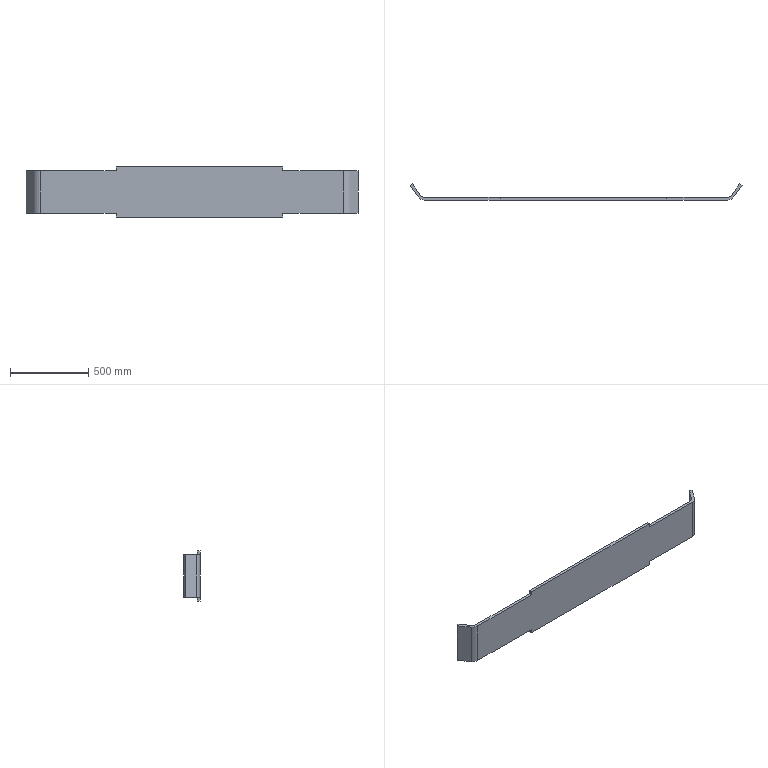Part | NX | features 后连杆右 2 | 1 solid | 22 faces | box 2121 x 103.15 x 320 mm | volume 11841435 mm3 | plane 18 | cylinder 4 | commonest cylinder face diameters 60 x2 96.74 x2
STEP:
#1=CARTESIAN_POINT('',(-191.209,-83.211,25.));
#2=VERTEX_POINT('',#1);
#3=CARTESIAN_POINT('',(-243.821,-10.798,25.));
#4=VERTEX_POINT('',#3);
#5=CARTESIAN_POINT('',(905.655,-1592.915,25.));
#6=DIRECTION('',(-0.5878,0.809,0.));
#7=VECTOR('',#6,1000.);
#8=LINE('',#5,#7);
#9=EDGE_CURVE('',#2,#4,#8,.T.);
#10=ORIENTED_EDGE('',*,*,#9,.F.);
#11=CARTESIAN_POINT('',(-191.209,-83.211,295.));
#12=VERTEX_POINT('',#11);
#13=CARTESIAN_POINT('',(-191.209,-83.211,320.));
#14=DIRECTION('',(0.,0.,-1.));
#15=VECTOR('',#14,1000.);
#16=LINE('',#13,#15);
#17=EDGE_CURVE('',#12,#2,#16,.T.);
#18=ORIENTED_EDGE('',*,*,#17,.F.);
#19=CARTESIAN_POINT('',(-243.821,-10.798,295.));
#20=VERTEX_POINT('',#19);
#21=CARTESIAN_POINT('',(905.655,-1592.915,295.));
#22=DIRECTION('',(0.5878,-0.809,0.));
#23=VECTOR('',#22,1000.);
#24=LINE('',#21,#23);
#25=EDGE_CURVE('',#20,#12,#24,.T.);
#26=ORIENTED_EDGE('',*,*,#25,.F.);
#27=CARTESIAN_POINT('',(-243.821,-10.798,320.));
#28=DIRECTION('',(0.,0.,-1.));
#29=VECTOR('',#28,1000.);
#30=LINE('',#27,#29);
#31=EDGE_CURVE('',#20,#4,#30,.T.);
#32=ORIENTED_EDGE('',*,*,#31,.T.);
#33=EDGE_LOOP('',(#10,#18,#26,#32));
#34=FACE_BOUND('',#33,.T.);
#35=CARTESIAN_POINT('',(905.655,-1592.915,320.));
#36=DIRECTION('',(-0.809,-0.5878,0.));
#37=DIRECTION('',(0.5878,-0.809,0.));
#38=AXIS2_PLACEMENT_3D('',#35,#36,#37);
#39=PLANE('',#38);
#40=ADVANCED_FACE('',(#34),#39,.T.);
#41=ORIENTED_EDGE('',*,*,#17,.T.);
#42=CARTESIAN_POINT('',(-152.077,-103.15,25.));
#43=VERTEX_POINT('',#42);
#44=CARTESIAN_POINT('',(-152.077,-54.78,25.));
#45=DIRECTION('',(0.,0.,1.));
#46=DIRECTION('',(1.,0.,0.));
#47=AXIS2_PLACEMENT_3D('',#44,#45,#46);
#48=CIRCLE('',#47,48.37);
#49=EDGE_CURVE('',#2,#43,#48,.T.);
#50=ORIENTED_EDGE('',*,*,#49,.T.);
#51=CARTESIAN_POINT('',(-152.077,-103.15,295.));
#52=VERTEX_POINT('',#51);
#53=CARTESIAN_POINT('',(-152.077,-103.15,320.));
#54=DIRECTION('',(0.,0.,-1.));
#55=VECTOR('',#54,1000.);
#56=LINE('',#53,#55);
#57=EDGE_CURVE('',#52,#43,#56,.T.);
#58=ORIENTED_EDGE('',*,*,#57,.F.);
#59=CARTESIAN_POINT('',(-152.077,-54.78,295.));
#60=DIRECTION('',(0.,0.,-1.));
#61=DIRECTION('',(-1.,0.,0.));
#62=AXIS2_PLACEMENT_3D('',#59,#60,#61);
#63=CIRCLE('',#62,48.37);
#64=EDGE_CURVE('',#52,#12,#63,.T.);
#65=ORIENTED_EDGE('',*,*,#64,.T.);
#66=EDGE_LOOP('',(#41,#50,#58,#65));
#67=FACE_BOUND('',#66,.T.);
#68=CARTESIAN_POINT('',(-152.077,-54.78,320.));
#69=DIRECTION('',(0.,0.,-1.));
#70=DIRECTION('',(-1.,0.,0.));
#71=AXIS2_PLACEMENT_3D('',#68,#69,#70);
#72=CYLINDRICAL_SURFACE('',#71,48.37);
#73=ADVANCED_FACE('',(#67),#72,.T.);
#74=CARTESIAN_POINT('',(331.828,-103.15,25.));
#75=VERTEX_POINT('',#74);
#76=CARTESIAN_POINT('',(816.627,-103.15,25.));
#77=DIRECTION('',(1.,0.,0.));
#78=VECTOR('',#77,1000.);
#79=LINE('',#76,#78);
#80=EDGE_CURVE('',#43,#75,#79,.T.);
#81=ORIENTED_EDGE('',*,*,#80,.T.);
#82=CARTESIAN_POINT('',(331.828,-103.15,0.));
#83=VERTEX_POINT('',#82);
#84=CARTESIAN_POINT('',(331.828,-103.15,320.));
#85=DIRECTION('',(0.,0.,-1.));
#86=VECTOR('',#85,1000.);
#87=LINE('',#84,#86);
#88=EDGE_CURVE('',#75,#83,#87,.T.);
#89=ORIENTED_EDGE('',*,*,#88,.T.);
#90=CARTESIAN_POINT('',(1396.426,-103.15,0.));
#91=VERTEX_POINT('',#90);
#92=CARTESIAN_POINT('',(816.627,-103.15,0.));
#93=DIRECTION('',(1.,0.,0.));
#94=VECTOR('',#93,1000.);
#95=LINE('',#92,#94);
#96=EDGE_CURVE('',#83,#91,#95,.T.);
#97=ORIENTED_EDGE('',*,*,#96,.T.);
#98=CARTESIAN_POINT('',(1396.426,-103.15,25.));
#99=VERTEX_POINT('',#98);
#100=CARTESIAN_POINT('',(1396.426,-103.15,320.));
#101=DIRECTION('',(0.,0.,1.));
#102=VECTOR('',#101,1000.);
#103=LINE('',#100,#102);
#104=EDGE_CURVE('',#91,#99,#103,.T.);
#105=ORIENTED_EDGE('',*,*,#104,.T.);
#106=CARTESIAN_POINT('',(1785.331,-103.15,25.));
#107=VERTEX_POINT('',#106);
#108=CARTESIAN_POINT('',(816.627,-103.15,25.));
#109=DIRECTION('',(1.,0.,0.));
#110=VECTOR('',#109,1000.);
#111=LINE('',#108,#110);
#112=EDGE_CURVE('',#99,#107,#111,.T.);
#113=ORIENTED_EDGE('',*,*,#112,.T.);
#114=CARTESIAN_POINT('',(1785.331,-103.15,295.));
#115=VERTEX_POINT('',#114);
#116=CARTESIAN_POINT('',(1785.331,-103.15,320.));
#117=DIRECTION('',(0.,0.,-1.));
#118=VECTOR('',#117,1000.);
#119=LINE('',#116,#118);
#120=EDGE_CURVE('',#115,#107,#119,.T.);
#121=ORIENTED_EDGE('',*,*,#120,.F.);
#122=CARTESIAN_POINT('',(1396.426,-103.15,295.));
#123=VERTEX_POINT('',#122);
#124=CARTESIAN_POINT('',(816.627,-103.15,295.));
#125=DIRECTION('',(-1.,0.,0.));
#126=VECTOR('',#125,1000.);
#127=LINE('',#124,#126);
#128=EDGE_CURVE('',#115,#123,#127,.T.);
#129=ORIENTED_EDGE('',*,*,#128,.T.);
#130=CARTESIAN_POINT('',(1396.426,-103.15,320.));
#131=VERTEX_POINT('',#130);
#132=CARTESIAN_POINT('',(1396.426,-103.15,320.));
#133=DIRECTION('',(0.,0.,1.));
#134=VECTOR('',#133,1000.);
#135=LINE('',#132,#134);
#136=EDGE_CURVE('',#123,#131,#135,.T.);
#137=ORIENTED_EDGE('',*,*,#136,.T.);
#138=CARTESIAN_POINT('',(331.828,-103.15,320.));
#139=VERTEX_POINT('',#138);
#140=CARTESIAN_POINT('',(816.627,-103.15,320.));
#141=DIRECTION('',(1.,0.,0.));
#142=VECTOR('',#141,1000.);
#143=LINE('',#140,#142);
#144=EDGE_CURVE('',#139,#131,#143,.T.);
#145=ORIENTED_EDGE('',*,*,#144,.F.);
#146=CARTESIAN_POINT('',(331.828,-103.15,295.));
#147=VERTEX_POINT('',#146);
#148=CARTESIAN_POINT('',(331.828,-103.15,320.));
#149=DIRECTION('',(0.,0.,-1.));
#150=VECTOR('',#149,1000.);
#151=LINE('',#148,#150);
#152=EDGE_CURVE('',#139,#147,#151,.T.);
#153=ORIENTED_EDGE('',*,*,#152,.T.);
#154=CARTESIAN_POINT('',(816.627,-103.15,295.));
#155=DIRECTION('',(-1.,0.,0.));
#156=VECTOR('',#155,1000.);
#157=LINE('',#154,#156);
#158=EDGE_CURVE('',#147,#52,#157,.T.);
#159=ORIENTED_EDGE('',*,*,#158,.T.);
#160=ORIENTED_EDGE('',*,*,#57,.T.);
#161=EDGE_LOOP('',(#81,#89,#97,#105,#113,#121,#129,#137,#145,#153,#159,#160));
#162=FACE_BOUND('',#161,.T.);
#163=CARTESIAN_POINT('',(816.627,-103.15,320.));
#164=DIRECTION('',(0.,1.,0.));
#165=DIRECTION('',(-1.,0.,0.));
#166=AXIS2_PLACEMENT_3D('',#163,#164,#165);
#167=PLANE('',#166);
#168=ADVANCED_FACE('',(#162),#167,.F.);
#169=CARTESIAN_POINT('',(1824.464,-83.211,25.));
#170=VERTEX_POINT('',#169);
#171=CARTESIAN_POINT('',(1785.331,-54.78,25.));
#172=DIRECTION('',(0.,0.,1.));
#173=DIRECTION('',(1.,0.,0.));
#174=AXIS2_PLACEMENT_3D('',#171,#172,#173);
#175=CIRCLE('',#174,48.37);
#176=EDGE_CURVE('',#170,#107,#175,.F.);
#177=ORIENTED_EDGE('',*,*,#176,.F.);
#178=CARTESIAN_POINT('',(1824.464,-83.211,295.));
#179=VERTEX_POINT('',#178);
#180=CARTESIAN_POINT('',(1824.464,-83.211,320.));
#181=DIRECTION('',(0.,0.,-1.));
#182=VECTOR('',#181,1000.);
#183=LINE('',#180,#182);
#184=EDGE_CURVE('',#179,#170,#183,.T.);
#185=ORIENTED_EDGE('',*,*,#184,.F.);
#186=CARTESIAN_POINT('',(1785.331,-54.78,295.));
#187=DIRECTION('',(0.,0.,-1.));
#188=DIRECTION('',(-1.,0.,0.));
#189=AXIS2_PLACEMENT_3D('',#186,#187,#188);
#190=CIRCLE('',#189,48.37);
#191=EDGE_CURVE('',#115,#179,#190,.F.);
#192=ORIENTED_EDGE('',*,*,#191,.F.);
#193=ORIENTED_EDGE('',*,*,#120,.T.);
#194=EDGE_LOOP('',(#177,#185,#192,#193));
#195=FACE_BOUND('',#194,.T.);
#196=CARTESIAN_POINT('',(1785.331,-54.78,320.));
#197=DIRECTION('',(0.,0.,-1.));
#198=DIRECTION('',(-1.,0.,0.));
#199=AXIS2_PLACEMENT_3D('',#196,#197,#198);
#200=CYLINDRICAL_SURFACE('',#199,48.37);
#201=ADVANCED_FACE('',(#195),#200,.T.);
#202=ORIENTED_EDGE('',*,*,#184,.T.);
#203=CARTESIAN_POINT('',(1877.075,-10.798,25.));
#204=VERTEX_POINT('',#203);
#205=CARTESIAN_POINT('',(727.6,-1592.915,25.));
#206=DIRECTION('',(0.5878,0.809,0.));
#207=VECTOR('',#206,1000.);
#208=LINE('',#205,#207);
#209=EDGE_CURVE('',#170,#204,#208,.T.);
#210=ORIENTED_EDGE('',*,*,#209,.T.);
#211=CARTESIAN_POINT('',(1877.075,-10.798,295.));
#212=VERTEX_POINT('',#211);
#213=CARTESIAN_POINT('',(1877.075,-10.798,320.));
#214=DIRECTION('',(0.,0.,-1.));
#215=VECTOR('',#214,1000.);
#216=LINE('',#213,#215);
#217=EDGE_CURVE('',#212,#204,#216,.T.);
#218=ORIENTED_EDGE('',*,*,#217,.F.);
#219=CARTESIAN_POINT('',(727.6,-1592.915,295.));
#220=DIRECTION('',(-0.5878,-0.809,0.));
#221=VECTOR('',#220,1000.);
#222=LINE('',#219,#221);
#223=EDGE_CURVE('',#212,#179,#222,.T.);
#224=ORIENTED_EDGE('',*,*,#223,.T.);
#225=EDGE_LOOP('',(#202,#210,#218,#224));
#226=FACE_BOUND('',#225,.T.);
#227=CARTESIAN_POINT('',(727.6,-1592.915,320.));
#228=DIRECTION('',(-0.809,0.5878,0.));
#229=DIRECTION('',(-0.5878,-0.809,0.));
#230=AXIS2_PLACEMENT_3D('',#227,#228,#229);
#231=PLANE('',#230);
#232=ADVANCED_FACE('',(#226),#231,.F.);
#233=ORIENTED_EDGE('',*,*,#217,.T.);
#234=CARTESIAN_POINT('',(1862.213,0.,25.));
#235=VERTEX_POINT('',#234);
#236=CARTESIAN_POINT('',(1966.103,-75.48,25.));
#237=DIRECTION('',(-0.809,0.5878,0.));
#238=VECTOR('',#237,1000.);
#239=LINE('',#236,#238);
#240=EDGE_CURVE('',#204,#235,#239,.T.);
#241=ORIENTED_EDGE('',*,*,#240,.T.);
#242=CARTESIAN_POINT('',(1862.213,0.,295.));
#243=VERTEX_POINT('',#242);
#244=CARTESIAN_POINT('',(1862.213,0.,320.));
#245=DIRECTION('',(0.,0.,-1.));
#246=VECTOR('',#245,1000.);
#247=LINE('',#244,#246);
#248=EDGE_CURVE('',#243,#235,#247,.T.);
#249=ORIENTED_EDGE('',*,*,#248,.F.);
#250=CARTESIAN_POINT('',(1966.103,-75.48,295.));
#251=DIRECTION('',(0.809,-0.5878,0.));
#252=VECTOR('',#251,1000.);
#253=LINE('',#250,#252);
#254=EDGE_CURVE('',#243,#212,#253,.T.);
#255=ORIENTED_EDGE('',*,*,#254,.T.);
#256=EDGE_LOOP('',(#233,#241,#249,#255));
#257=FACE_BOUND('',#256,.T.);
#258=CARTESIAN_POINT('',(1966.103,-75.48,320.));
#259=DIRECTION('',(-0.5878,-0.809,0.));
#260=DIRECTION('',(0.809,-0.5878,0.));
#261=AXIS2_PLACEMENT_3D('',#258,#259,#260);
#262=PLANE('',#261);
#263=ADVANCED_FACE('',(#257),#262,.F.);
#264=CARTESIAN_POINT('',(1809.602,-72.414,25.));
#265=VERTEX_POINT('',#264);
#266=CARTESIAN_POINT('',(712.738,-1582.117,25.));
#267=DIRECTION('',(0.5878,0.809,0.));
#268=VECTOR('',#267,1000.);
#269=LINE('',#266,#268);
#270=EDGE_CURVE('',#265,#235,#269,.T.);
#271=ORIENTED_EDGE('',*,*,#270,.F.);
#272=CARTESIAN_POINT('',(1809.602,-72.414,295.));
#273=VERTEX_POINT('',#272);
#274=CARTESIAN_POINT('',(1809.602,-72.414,320.));
#275=DIRECTION('',(0.,0.,-1.));
#276=VECTOR('',#275,1000.);
#277=LINE('',#274,#276);
#278=EDGE_CURVE('',#273,#265,#277,.T.);
#279=ORIENTED_EDGE('',*,*,#278,.F.);
#280=CARTESIAN_POINT('',(712.738,-1582.117,295.));
#281=DIRECTION('',(-0.5878,-0.809,0.));
#282=VECTOR('',#281,1000.);
#283=LINE('',#280,#282);
#284=EDGE_CURVE('',#243,#273,#283,.T.);
#285=ORIENTED_EDGE('',*,*,#284,.F.);
#286=ORIENTED_EDGE('',*,*,#248,.T.);
#287=EDGE_LOOP('',(#271,#279,#285,#286));
#288=FACE_BOUND('',#287,.T.);
#289=CARTESIAN_POINT('',(712.738,-1582.117,320.));
#290=DIRECTION('',(-0.809,0.5878,0.));
#291=DIRECTION('',(-0.5878,-0.809,0.));
#292=AXIS2_PLACEMENT_3D('',#289,#290,#291);
#293=PLANE('',#292);
#294=ADVANCED_FACE('',(#288),#293,.T.);
#295=ORIENTED_EDGE('',*,*,#278,.T.);
#296=CARTESIAN_POINT('',(1785.331,-84.78,25.));
#297=VERTEX_POINT('',#296);
#298=CARTESIAN_POINT('',(1785.331,-54.78,25.));
#299=DIRECTION('',(0.,0.,1.));
#300=DIRECTION('',(1.,0.,0.));
#301=AXIS2_PLACEMENT_3D('',#298,#299,#300);
#302=CIRCLE('',#301,30.);
#303=EDGE_CURVE('',#265,#297,#302,.F.);
#304=ORIENTED_EDGE('',*,*,#303,.T.);
#305=CARTESIAN_POINT('',(1785.331,-84.78,295.));
#306=VERTEX_POINT('',#305);
#307=CARTESIAN_POINT('',(1785.331,-84.78,320.));
#308=DIRECTION('',(0.,0.,-1.));
#309=VECTOR('',#308,1000.);
#310=LINE('',#307,#309);
#311=EDGE_CURVE('',#306,#297,#310,.T.);
#312=ORIENTED_EDGE('',*,*,#311,.F.);
#313=CARTESIAN_POINT('',(1785.331,-54.78,295.));
#314=DIRECTION('',(0.,0.,-1.));
#315=DIRECTION('',(-1.,0.,0.));
#316=AXIS2_PLACEMENT_3D('',#313,#314,#315);
#317=CIRCLE('',#316,30.);
#318=EDGE_CURVE('',#306,#273,#317,.F.);
#319=ORIENTED_EDGE('',*,*,#318,.T.);
#320=EDGE_LOOP('',(#295,#304,#312,#319));
#321=FACE_BOUND('',#320,.T.);
#322=CARTESIAN_POINT('',(1785.331,-54.78,320.));
#323=DIRECTION('',(0.,0.,-1.));
#324=DIRECTION('',(-1.,0.,0.));
#325=AXIS2_PLACEMENT_3D('',#322,#323,#324);
#326=CYLINDRICAL_SURFACE('',#325,30.);
#327=ADVANCED_FACE('',(#321),#326,.F.);
#328=CARTESIAN_POINT('',(331.828,-84.78,25.));
#329=VERTEX_POINT('',#328);
#330=CARTESIAN_POINT('',(331.828,-84.78,0.));
#331=VERTEX_POINT('',#330);
#332=CARTESIAN_POINT('',(331.828,-84.78,320.));
#333=DIRECTION('',(0.,0.,-1.));
#334=VECTOR('',#333,1000.);
#335=LINE('',#332,#334);
#336=EDGE_CURVE('',#329,#331,#335,.T.);
#337=ORIENTED_EDGE('',*,*,#336,.F.);
#338=CARTESIAN_POINT('',(-152.077,-84.78,25.));
#339=VERTEX_POINT('',#338);
#340=CARTESIAN_POINT('',(816.627,-84.78,25.));
#341=DIRECTION('',(1.,0.,0.));
#342=VECTOR('',#341,1000.);
#343=LINE('',#340,#342);
#344=EDGE_CURVE('',#339,#329,#343,.T.);
#345=ORIENTED_EDGE('',*,*,#344,.F.);
#346=CARTESIAN_POINT('',(-152.077,-84.78,295.));
#347=VERTEX_POINT('',#346);
#348=CARTESIAN_POINT('',(-152.077,-84.78,320.));
#349=DIRECTION('',(0.,0.,-1.));
#350=VECTOR('',#349,1000.);
#351=LINE('',#348,#350);
#352=EDGE_CURVE('',#347,#339,#351,.T.);
#353=ORIENTED_EDGE('',*,*,#352,.F.);
#354=CARTESIAN_POINT('',(331.828,-84.78,295.));
#355=VERTEX_POINT('',#354);
#356=CARTESIAN_POINT('',(816.627,-84.78,295.));
#357=DIRECTION('',(-1.,0.,0.));
#358=VECTOR('',#357,1000.);
#359=LINE('',#356,#358);
#360=EDGE_CURVE('',#355,#347,#359,.T.);
#361=ORIENTED_EDGE('',*,*,#360,.F.);
#362=CARTESIAN_POINT('',(331.828,-84.78,320.));
#363=VERTEX_POINT('',#362);
#364=CARTESIAN_POINT('',(331.828,-84.78,320.));
#365=DIRECTION('',(0.,0.,-1.));
#366=VECTOR('',#365,1000.);
#367=LINE('',#364,#366);
#368=EDGE_CURVE('',#363,#355,#367,.T.);
#369=ORIENTED_EDGE('',*,*,#368,.F.);
#370=CARTESIAN_POINT('',(1396.426,-84.78,320.));
#371=VERTEX_POINT('',#370);
#372=CARTESIAN_POINT('',(816.627,-84.78,320.));
#373=DIRECTION('',(1.,0.,0.));
#374=VECTOR('',#373,1000.);
#375=LINE('',#372,#374);
#376=EDGE_CURVE('',#363,#371,#375,.T.);
#377=ORIENTED_EDGE('',*,*,#376,.T.);
#378=CARTESIAN_POINT('',(1396.426,-84.78,295.));
#379=VERTEX_POINT('',#378);
#380=CARTESIAN_POINT('',(1396.426,-84.78,320.));
#381=DIRECTION('',(0.,0.,1.));
#382=VECTOR('',#381,1000.);
#383=LINE('',#380,#382);
#384=EDGE_CURVE('',#379,#371,#383,.T.);
#385=ORIENTED_EDGE('',*,*,#384,.F.);
#386=CARTESIAN_POINT('',(816.627,-84.78,295.));
#387=DIRECTION('',(-1.,0.,0.));
#388=VECTOR('',#387,1000.);
#389=LINE('',#386,#388);
#390=EDGE_CURVE('',#306,#379,#389,.T.);
#391=ORIENTED_EDGE('',*,*,#390,.F.);
#392=ORIENTED_EDGE('',*,*,#311,.T.);
#393=CARTESIAN_POINT('',(1396.426,-84.78,25.));
#394=VERTEX_POINT('',#393);
#395=CARTESIAN_POINT('',(816.627,-84.78,25.));
#396=DIRECTION('',(1.,0.,0.));
#397=VECTOR('',#396,1000.);
#398=LINE('',#395,#397);
#399=EDGE_CURVE('',#394,#297,#398,.T.);
#400=ORIENTED_EDGE('',*,*,#399,.F.);
#401=CARTESIAN_POINT('',(1396.426,-84.78,0.));
#402=VERTEX_POINT('',#401);
#403=CARTESIAN_POINT('',(1396.426,-84.78,320.));
#404=DIRECTION('',(0.,0.,1.));
#405=VECTOR('',#404,1000.);
#406=LINE('',#403,#405);
#407=EDGE_CURVE('',#402,#394,#406,.T.);
#408=ORIENTED_EDGE('',*,*,#407,.F.);
#409=CARTESIAN_POINT('',(816.627,-84.78,0.));
#410=DIRECTION('',(1.,0.,0.));
#411=VECTOR('',#410,1000.);
#412=LINE('',#409,#411);
#413=EDGE_CURVE('',#331,#402,#412,.T.);
#414=ORIENTED_EDGE('',*,*,#413,.F.);
#415=EDGE_LOOP('',(#337,#345,#353,#361,#369,#377,#385,#391,#392,#400,#408,#414));
#416=FACE_BOUND('',#415,.T.);
#417=CARTESIAN_POINT('',(816.627,-84.78,320.));
#418=DIRECTION('',(0.,1.,0.));
#419=DIRECTION('',(0.,0.,1.));
#420=AXIS2_PLACEMENT_3D('',#417,#418,#419);
#421=PLANE('',#420);
#422=ADVANCED_FACE('',(#416),#421,.T.);
#423=CARTESIAN_POINT('',(-176.348,-72.414,25.));
#424=VERTEX_POINT('',#423);
#425=CARTESIAN_POINT('',(-152.077,-54.78,25.));
#426=DIRECTION('',(0.,0.,1.));
#427=DIRECTION('',(1.,0.,0.));
#428=AXIS2_PLACEMENT_3D('',#425,#426,#427);
#429=CIRCLE('',#428,30.);
#430=EDGE_CURVE('',#424,#339,#429,.T.);
#431=ORIENTED_EDGE('',*,*,#430,.F.);
#432=CARTESIAN_POINT('',(-176.348,-72.414,295.));
#433=VERTEX_POINT('',#432);
#434=CARTESIAN_POINT('',(-176.348,-72.414,320.));
#435=DIRECTION('',(0.,0.,-1.));
#436=VECTOR('',#435,1000.);
#437=LINE('',#434,#436);
#438=EDGE_CURVE('',#433,#424,#437,.T.);
#439=ORIENTED_EDGE('',*,*,#438,.F.);
#440=CARTESIAN_POINT('',(-152.077,-54.78,295.));
#441=DIRECTION('',(0.,0.,-1.));
#442=DIRECTION('',(-1.,0.,0.));
#443=AXIS2_PLACEMENT_3D('',#440,#441,#442);
#444=CIRCLE('',#443,30.);
#445=EDGE_CURVE('',#347,#433,#444,.T.);
#446=ORIENTED_EDGE('',*,*,#445,.F.);
#447=ORIENTED_EDGE('',*,*,#352,.T.);
#448=EDGE_LOOP('',(#431,#439,#446,#447));
#449=FACE_BOUND('',#448,.T.);
#450=CARTESIAN_POINT('',(-152.077,-54.78,320.));
#451=DIRECTION('',(0.,0.,-1.));
#452=DIRECTION('',(-1.,0.,0.));
#453=AXIS2_PLACEMENT_3D('',#450,#451,#452);
#454=CYLINDRICAL_SURFACE('',#453,30.);
#455=ADVANCED_FACE('',(#449),#454,.F.);
#456=ORIENTED_EDGE('',*,*,#438,.T.);
#457=CARTESIAN_POINT('',(-228.959,0.,25.));
#458=VERTEX_POINT('',#457);
#459=CARTESIAN_POINT('',(920.516,-1582.117,25.));
#460=DIRECTION('',(-0.5878,0.809,0.));
#461=VECTOR('',#460,1000.);
#462=LINE('',#459,#461);
#463=EDGE_CURVE('',#424,#458,#462,.T.);
#464=ORIENTED_EDGE('',*,*,#463,.T.);
#465=CARTESIAN_POINT('',(-228.959,0.,295.));
#466=VERTEX_POINT('',#465);
#467=CARTESIAN_POINT('',(-228.959,0.,320.));
#468=DIRECTION('',(0.,0.,-1.));
#469=VECTOR('',#468,1000.);
#470=LINE('',#467,#469);
#471=EDGE_CURVE('',#466,#458,#470,.T.);
#472=ORIENTED_EDGE('',*,*,#471,.F.);
#473=CARTESIAN_POINT('',(920.516,-1582.117,295.));
#474=DIRECTION('',(0.5878,-0.809,0.));
#475=VECTOR('',#474,1000.);
#476=LINE('',#473,#475);
#477=EDGE_CURVE('',#466,#433,#476,.T.);
#478=ORIENTED_EDGE('',*,*,#477,.T.);
#479=EDGE_LOOP('',(#456,#464,#472,#478));
#480=FACE_BOUND('',#479,.T.);
#481=CARTESIAN_POINT('',(920.516,-1582.117,320.));
#482=DIRECTION('',(-0.809,-0.5878,0.));
#483=DIRECTION('',(0.5878,-0.809,0.));
#484=AXIS2_PLACEMENT_3D('',#481,#482,#483);
#485=PLANE('',#484);
#486=ADVANCED_FACE('',(#480),#485,.F.);
#487=CARTESIAN_POINT('',(-332.848,-75.48,25.));
#488=DIRECTION('',(0.809,0.5878,0.));
#489=VECTOR('',#488,1000.);
#490=LINE('',#487,#489);
#491=EDGE_CURVE('',#4,#458,#490,.T.);
#492=ORIENTED_EDGE('',*,*,#491,.F.);
#493=ORIENTED_EDGE('',*,*,#31,.F.);
#494=CARTESIAN_POINT('',(-332.848,-75.48,295.));
#495=DIRECTION('',(-0.809,-0.5878,0.));
#496=VECTOR('',#495,1000.);
#497=LINE('',#494,#496);
#498=EDGE_CURVE('',#466,#20,#497,.T.);
#499=ORIENTED_EDGE('',*,*,#498,.F.);
#500=ORIENTED_EDGE('',*,*,#471,.T.);
#501=EDGE_LOOP('',(#492,#493,#499,#500));
#502=FACE_BOUND('',#501,.T.);
#503=CARTESIAN_POINT('',(-332.848,-75.48,320.));
#504=DIRECTION('',(-0.5878,0.809,0.));
#505=DIRECTION('',(-0.809,-0.5878,0.));
#506=AXIS2_PLACEMENT_3D('',#503,#504,#505);
#507=PLANE('',#506);
#508=ADVANCED_FACE('',(#502),#507,.T.);
#509=CARTESIAN_POINT('',(331.828,-1657.597,320.));
#510=DIRECTION('',(0.,1.,0.));
#511=VECTOR('',#510,1000.);
#512=LINE('',#509,#511);
#513=EDGE_CURVE('',#139,#363,#512,.T.);
#514=ORIENTED_EDGE('',*,*,#513,.F.);
#515=ORIENTED_EDGE('',*,*,#144,.T.);
#516=CARTESIAN_POINT('',(1396.426,-1657.597,320.));
#517=DIRECTION('',(0.,-1.,0.));
#518=VECTOR('',#517,1000.);
#519=LINE('',#516,#518);
#520=EDGE_CURVE('',#371,#131,#519,.T.);
#521=ORIENTED_EDGE('',*,*,#520,.F.);
#522=ORIENTED_EDGE('',*,*,#376,.F.);
#523=EDGE_LOOP('',(#514,#515,#521,#522));
#524=FACE_BOUND('',#523,.T.);
#525=CARTESIAN_POINT('',(816.627,-1657.597,320.));
#526=DIRECTION('',(0.,0.,1.));
#527=DIRECTION('',(1.,0.,0.));
#528=AXIS2_PLACEMENT_3D('',#525,#526,#527);
#529=PLANE('',#528);
#530=ADVANCED_FACE('',(#524),#529,.T.);
#531=ORIENTED_EDGE('',*,*,#96,.F.);
#532=CARTESIAN_POINT('',(331.828,-1657.597,0.));
#533=DIRECTION('',(0.,1.,0.));
#534=VECTOR('',#533,1000.);
#535=LINE('',#532,#534);
#536=EDGE_CURVE('',#83,#331,#535,.T.);
#537=ORIENTED_EDGE('',*,*,#536,.T.);
#538=ORIENTED_EDGE('',*,*,#413,.T.);
#539=CARTESIAN_POINT('',(1396.426,-1657.597,0.));
#540=DIRECTION('',(0.,-1.,0.));
#541=VECTOR('',#540,1000.);
#542=LINE('',#539,#541);
#543=EDGE_CURVE('',#402,#91,#542,.T.);
#544=ORIENTED_EDGE('',*,*,#543,.T.);
#545=EDGE_LOOP('',(#531,#537,#538,#544));
#546=FACE_BOUND('',#545,.T.);
#547=CARTESIAN_POINT('',(816.627,-1657.597,0.));
#548=DIRECTION('',(0.,0.,1.));
#549=DIRECTION('',(1.,0.,0.));
#550=AXIS2_PLACEMENT_3D('',#547,#548,#549);
#551=PLANE('',#550);
#552=ADVANCED_FACE('',(#546),#551,.F.);
#553=CARTESIAN_POINT('',(1396.426,-160.,25.));
#554=DIRECTION('',(0.,1.,0.));
#555=VECTOR('',#554,1000.);
#556=LINE('',#553,#555);
#557=EDGE_CURVE('',#99,#394,#556,.T.);
#558=ORIENTED_EDGE('',*,*,#557,.T.);
#559=ORIENTED_EDGE('',*,*,#399,.T.);
#560=ORIENTED_EDGE('',*,*,#303,.F.);
#561=ORIENTED_EDGE('',*,*,#270,.T.);
#562=ORIENTED_EDGE('',*,*,#240,.F.);
#563=ORIENTED_EDGE('',*,*,#209,.F.);
#564=ORIENTED_EDGE('',*,*,#176,.T.);
#565=ORIENTED_EDGE('',*,*,#112,.F.);
#566=EDGE_LOOP('',(#558,#559,#560,#561,#562,#563,#564,#565));
#567=FACE_BOUND('',#566,.T.);
#568=CARTESIAN_POINT('',(1972.075,-160.,25.));
#569=DIRECTION('',(0.,0.,1.));
#570=DIRECTION('',(1.,0.,0.));
#571=AXIS2_PLACEMENT_3D('',#568,#569,#570);
#572=PLANE('',#571);
#573=ADVANCED_FACE('',(#567),#572,.F.);
#574=ORIENTED_EDGE('',*,*,#543,.F.);
#575=ORIENTED_EDGE('',*,*,#407,.T.);
#576=ORIENTED_EDGE('',*,*,#557,.F.);
#577=ORIENTED_EDGE('',*,*,#104,.F.);
#578=EDGE_LOOP('',(#574,#575,#576,#577));
#579=FACE_BOUND('',#578,.T.);
#580=CARTESIAN_POINT('',(1396.426,-160.,0.));
#581=DIRECTION('',(-1.,0.,0.));
#582=DIRECTION('',(0.,-1.,0.));
#583=AXIS2_PLACEMENT_3D('',#580,#581,#582);
#584=PLANE('',#583);
#585=ADVANCED_FACE('',(#579),#584,.F.);
#586=ORIENTED_EDGE('',*,*,#49,.F.);
#587=ORIENTED_EDGE('',*,*,#9,.T.);
#588=ORIENTED_EDGE('',*,*,#491,.T.);
#589=ORIENTED_EDGE('',*,*,#463,.F.);
#590=ORIENTED_EDGE('',*,*,#430,.T.);
#591=ORIENTED_EDGE('',*,*,#344,.T.);
#592=CARTESIAN_POINT('',(331.828,-160.,25.));
#593=DIRECTION('',(0.,1.,0.));
#594=VECTOR('',#593,1000.);
#595=LINE('',#592,#594);
#596=EDGE_CURVE('',#75,#329,#595,.T.);
#597=ORIENTED_EDGE('',*,*,#596,.F.);
#598=ORIENTED_EDGE('',*,*,#80,.F.);
#599=EDGE_LOOP('',(#586,#587,#588,#589,#590,#591,#597,#598));
#600=FACE_BOUND('',#599,.T.);
#601=CARTESIAN_POINT('',(-243.821,-160.,25.));
#602=DIRECTION('',(0.,0.,1.));
#603=DIRECTION('',(1.,0.,0.));
#604=AXIS2_PLACEMENT_3D('',#601,#602,#603);
#605=PLANE('',#604);
#606=ADVANCED_FACE('',(#600),#605,.F.);
#607=ORIENTED_EDGE('',*,*,#596,.T.);
#608=ORIENTED_EDGE('',*,*,#336,.T.);
#609=ORIENTED_EDGE('',*,*,#536,.F.);
#610=ORIENTED_EDGE('',*,*,#88,.F.);
#611=EDGE_LOOP('',(#607,#608,#609,#610));
#612=FACE_BOUND('',#611,.T.);
#613=CARTESIAN_POINT('',(331.828,-160.,0.));
#614=DIRECTION('',(1.,0.,0.));
#615=DIRECTION('',(0.,1.,0.));
#616=AXIS2_PLACEMENT_3D('',#613,#614,#615);
#617=PLANE('',#616);
#618=ADVANCED_FACE('',(#612),#617,.F.);
#619=ORIENTED_EDGE('',*,*,#191,.T.);
#620=ORIENTED_EDGE('',*,*,#223,.F.);
#621=ORIENTED_EDGE('',*,*,#254,.F.);
#622=ORIENTED_EDGE('',*,*,#284,.T.);
#623=ORIENTED_EDGE('',*,*,#318,.F.);
#624=ORIENTED_EDGE('',*,*,#390,.T.);
#625=CARTESIAN_POINT('',(1396.426,-160.,295.));
#626=DIRECTION('',(0.,1.,0.));
#627=VECTOR('',#626,1000.);
#628=LINE('',#625,#627);
#629=EDGE_CURVE('',#123,#379,#628,.T.);
#630=ORIENTED_EDGE('',*,*,#629,.F.);
#631=ORIENTED_EDGE('',*,*,#128,.F.);
#632=EDGE_LOOP('',(#619,#620,#621,#622,#623,#624,#630,#631));
#633=FACE_BOUND('',#632,.T.);
#634=CARTESIAN_POINT('',(1972.075,-160.,295.));
#635=DIRECTION('',(0.,0.,-1.));
#636=DIRECTION('',(-1.,0.,0.));
#637=AXIS2_PLACEMENT_3D('',#634,#635,#636);
#638=PLANE('',#637);
#639=ADVANCED_FACE('',(#633),#638,.F.);
#640=ORIENTED_EDGE('',*,*,#629,.T.);
#641=ORIENTED_EDGE('',*,*,#384,.T.);
#642=ORIENTED_EDGE('',*,*,#520,.T.);
#643=ORIENTED_EDGE('',*,*,#136,.F.);
#644=EDGE_LOOP('',(#640,#641,#642,#643));
#645=FACE_BOUND('',#644,.T.);
#646=CARTESIAN_POINT('',(1396.426,-160.,320.));
#647=DIRECTION('',(-1.,0.,0.));
#648=DIRECTION('',(0.,-1.,0.));
#649=AXIS2_PLACEMENT_3D('',#646,#647,#648);
#650=PLANE('',#649);
#651=ADVANCED_FACE('',(#645),#650,.F.);
#652=CARTESIAN_POINT('',(331.828,-160.,295.));
#653=DIRECTION('',(0.,1.,0.));
#654=VECTOR('',#653,1000.);
#655=LINE('',#652,#654);
#656=EDGE_CURVE('',#147,#355,#655,.T.);
#657=ORIENTED_EDGE('',*,*,#656,.T.);
#658=ORIENTED_EDGE('',*,*,#360,.T.);
#659=ORIENTED_EDGE('',*,*,#445,.T.);
#660=ORIENTED_EDGE('',*,*,#477,.F.);
#661=ORIENTED_EDGE('',*,*,#498,.T.);
#662=ORIENTED_EDGE('',*,*,#25,.T.);
#663=ORIENTED_EDGE('',*,*,#64,.F.);
#664=ORIENTED_EDGE('',*,*,#158,.F.);
#665=EDGE_LOOP('',(#657,#658,#659,#660,#661,#662,#663,#664));
#666=FACE_BOUND('',#665,.T.);
#667=CARTESIAN_POINT('',(-243.821,-160.,295.));
#668=DIRECTION('',(0.,0.,-1.));
#669=DIRECTION('',(-1.,0.,0.));
#670=AXIS2_PLACEMENT_3D('',#667,#668,#669);
#671=PLANE('',#670);
#672=ADVANCED_FACE('',(#666),#671,.F.);
#673=ORIENTED_EDGE('',*,*,#513,.T.);
#674=ORIENTED_EDGE('',*,*,#368,.T.);
#675=ORIENTED_EDGE('',*,*,#656,.F.);
#676=ORIENTED_EDGE('',*,*,#152,.F.);
#677=EDGE_LOOP('',(#673,#674,#675,#676));
#678=FACE_BOUND('',#677,.T.);
#679=CARTESIAN_POINT('',(331.828,-160.,320.));
#680=DIRECTION('',(1.,0.,0.));
#681=DIRECTION('',(0.,1.,0.));
#682=AXIS2_PLACEMENT_3D('',#679,#680,#681);
#683=PLANE('',#682);
#684=ADVANCED_FACE('',(#678),#683,.F.);
#685=CLOSED_SHELL('',(#40,#73,#168,#201,#232,#263,#294,#327,#422,#455,#486,#508,#530,#552,#573,#585,#606,#618,#639,#651,#672,#684));
#686=MANIFOLD_SOLID_BREP('',#685);
#687=(LENGTH_UNIT()NAMED_UNIT(*)SI_UNIT(.MILLI.,.METRE.));
#688=UNCERTAINTY_MEASURE_WITH_UNIT(LENGTH_MEASURE(0.00001),#687,'','');
#689=(NAMED_UNIT(*)PLANE_ANGLE_UNIT()SI_UNIT($,.RADIAN.));
#690=(NAMED_UNIT(*)SI_UNIT($,.STERADIAN.)SOLID_ANGLE_UNIT());
#691=(GEOMETRIC_REPRESENTATION_CONTEXT(3)GLOBAL_UNCERTAINTY_ASSIGNED_CONTEXT((#688))GLOBAL_UNIT_ASSIGNED_CONTEXT((#687,#689,#690))REPRESENTATION_CONTEXT('',''));
#692=ADVANCED_BREP_SHAPE_REPRESENTATION('',(#686),#691);